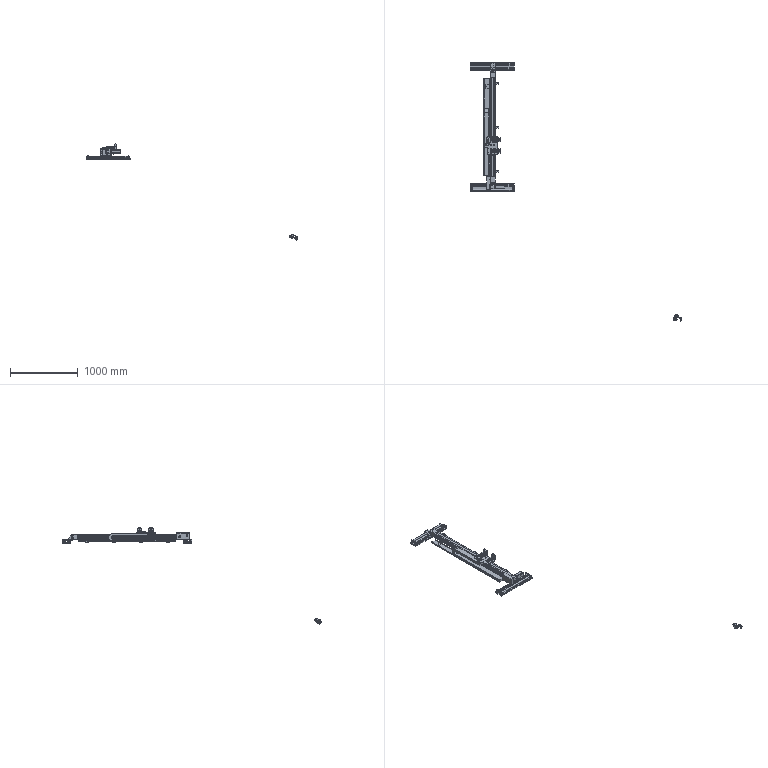Part | SolidWorks | features ReferencePattern 9, LocalLPattern 2, MirrorCompFeat 1 | 65 solids | 2955 faces | box 3126 x 3821 x 1424 mm | volume 19246728 mm3 | plane 1388 | cylinder 1313 | cone 234 | torus 12 | spline 8 | commonest cylinder face diameters 5 x135 7 x120 6 x76 0.4 x60 11 x60 9 x56